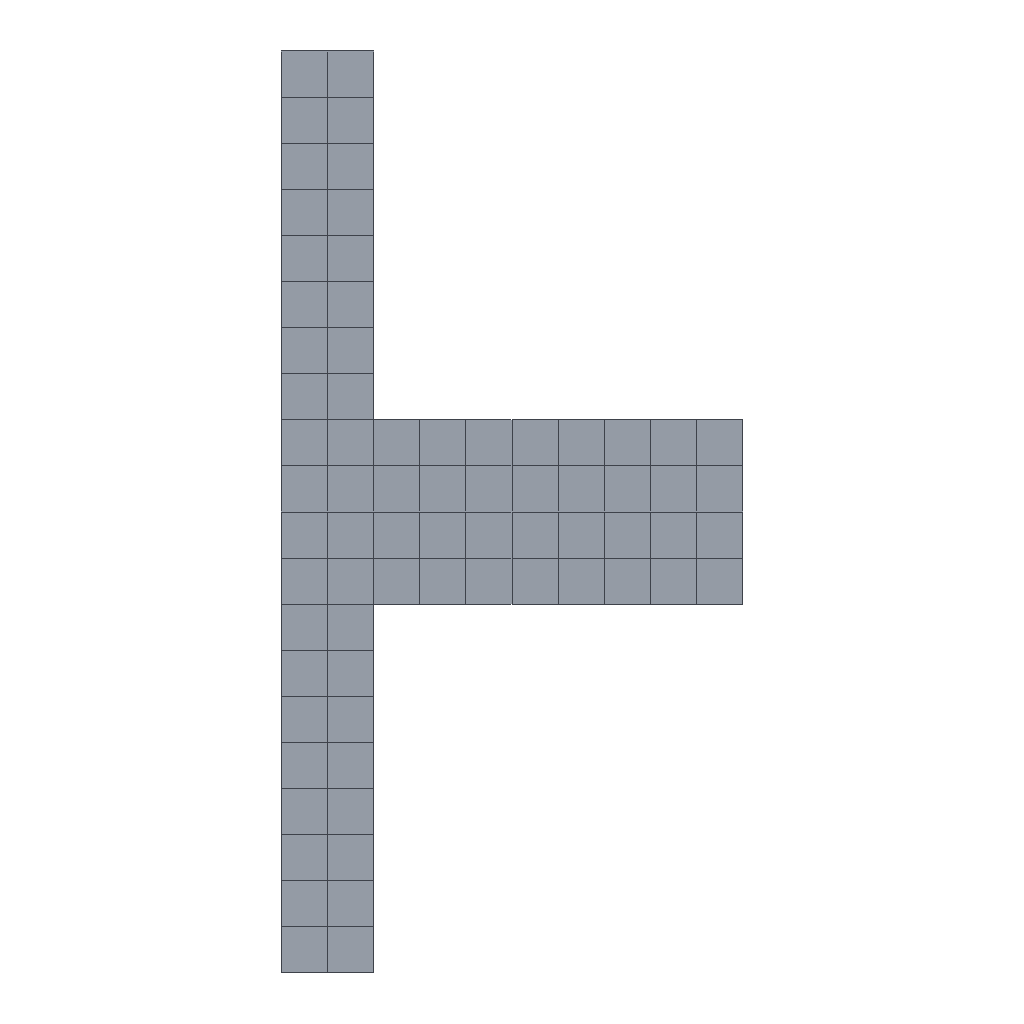Simulation study | abaqus
Set-up summary:
category,name,step,type,value,unit,region
solver,abaqus
solver,version,,,Abaqus/Standard 3DEXPERIENCE R2017x HotFix 2
units,not stated in the deck,,not stated
analysis,deck,,static,static
load_step,deadLoad,deadLoad,static
load_step,heat1,heat1,static
load_step,cool1,cool1,static
load_step,heat2,heat2,static
load_step,cool2,cool2,static
load_step,heat3,heat3,static
load_step,cool3,cool3,static
load_step,heat4,heat4,static
load_step,cool4,cool4,static
load_step,requested,,,9
mesh,nodes,,,114
mesh,elements,,,72
element_type,CAX4I,,axisymmetric,72
load,load commands in deck,,count,10
bc,support commands in deck,,count,2
material,STEEL,,in results
check,setup vs results,,match,"per instance, exact: element labels, types and connectivity; labels of the nodes the elements use; coordinates of those nodes at SINGLE_PRECISION in 2 of 2 instance(s)"
Abaqus input file, long lists of numbers shortened:
*Heading
** Job name: flange_kin Model name: flange_kin
** Generated by: Abaqus/CAE 2017.HF2
*Preprint, echo=NO, model=NO, history=NO, contact=NO
**
** PARTS
**
*Part, name=botFlange
*End Part
**
*Part, name=topFlange
*End Part
**
**
** ASSEMBLY
**
*Assembly, name=Assembly
**
*Instance, name=botFlange-1, part=botFlange
*Node
      1, 0.09, -0.02
      2,  0.13, -0.02
** (55 more lines like these left out)
*Element, type=CAX4I
1,  1, 10, 42,  4
2, 10, 11, 43, 42
** (34 more lines like these left out)
*Nset, nset=_PickedSet2, internal, generate
  1,  57,   1
*Elset, elset=_PickedSet2, internal, generate
  1,  36,   1
** Section: Section-1
*Solid Section, elset=_PickedSet2, material=steel
1.,
*End Instance
**
*Instance, name=topFlange-1, part=topFlange
*Node
      1, 0.09,           0.
      2,  0.13,           0.
** (55 more lines like these left out)
*Element, type=CAX4I
1,  1, 10, 42,  4
2, 10, 11, 43, 42
** (34 more lines like these left out)
*Nset, nset=_PickedSet2, internal, generate
  1,  57,   1
*Elset, elset=_PickedSet2, internal, generate
  1,  36,   1
** Section: Section-1
*Solid Section, elset=_PickedSet2, material=steel
1.,
*End Instance
**
*Nset, nset=all, instance=botFlange-1, generate
  1,  57,   1
*Nset, nset=all, instance=topFlange-1, generate
  1,  57,   1
*Elset, elset=all, instance=botFlange-1, generate
  1,  36,   1
*Elset, elset=all, instance=topFlange-1, generate
  1,  36,   1
*Nset, nset=botBolt, instance=botFlange-1
 4,
*Nset, nset=fix, instance=topFlange-1
 6,
*Nset, nset=topBolt, instance=topFlange-1
 4,
*Nset, nset=tops, instance=botFlange-1
  7,  8, 31
*Nset, nset=tops, instance=topFlange-1
  7,  8, 27
*Elset, elset=tops, instance=botFlange-1
 23, 24
*Elset, elset=tops, instance=topFlange-1
 26, 36
*Elset, elset=_botFlange_S3, internal, instance=botFlange-1
  5,  6,  7,  8, 31, 32, 33, 34, 35, 36
*Surface, type=ELEMENT, name=botFlange
_botFlange_S3, S3
*Elset, elset=_press_S3, internal, instance=botFlange-1
 23, 24
*Elset, elset=_press_S2, internal, instance=topFlange-1
 26, 36
*Surface, type=ELEMENT, name=press
_press_S3, S3
_press_S2, S2
*Elset, elset=_topFlange_S1, internal, instance=topFlange-1, generate
 1,  4,  1
*Elset, elset=_topFlange_S2, internal, instance=topFlange-1, generate
 10,  16,   2
*Elset, elset=_topFlange_S4, internal, instance=topFlange-1
 17, 27
*Surface, type=ELEMENT, name=topFlange
_topFlange_S1, S1
_topFlange_S2, S2
_topFlange_S4, S4
** Constraint: tie bolt 1
*Equation
2
topBolt, 1, 1.
botBolt, 1, -1.
** Constraint: tie bolt 2
*Equation
2
topBolt, 2, 1.
botBolt, 2, -1.
*End Assembly
**
** MATERIALS
**
*Material, name=steel
*Elastic
 2.10439e+11, 0.3
*Expansion
 2e-05,
*Plastic, hardening=KINEMATIC
     2e+08,      0.
 1.237e+09, 0.05411
**
** INTERACTION PROPERTIES
**
*Surface Interaction, name=fric
1.,
*Friction, slip tolerance=0.005
 0.1,
*Surface Behavior, pressure-overclosure=HARD
**
** INTERACTIONS
**
** Interaction: Int-1
*Contact Pair, interaction=fric, small sliding
topFlange, botFlange
** ----------------------------------------------------------------
**
** STEP: deadLoad
**
*Step, name=deadLoad, nlgeom=YES
apply dead load of pipe weight
*Static
0.1, 1., 1e-05, 1.
**
** BOUNDARY CONDITIONS
**
** Name: fixRB Type: Displacement/Rotation
*Boundary
fix, 2, 2
**
** LOADS
**
** Name: Load-1   Type: Pressure
*Dsload
press, P, -4.9735e+07
**
** PREDEFINED FIELDS
**
** Name: Field-1   Type: Temperature
*Temperature
all, 20.
**
** OUTPUT REQUESTS
**
*Restart, write, frequency=0
**
** FIELD OUTPUT: F-Output-1
**
*Output, field, variable=PRESELECT
**
** HISTORY OUTPUT: H-Output-1
**
*Output, history, variable=PRESELECT
*End Step
** ----------------------------------------------------------------
**
** STEP: heat1
**
*Step, name=heat1, nlgeom=YES
1st heat up cycle
*Static
0.05, 1., 1e-05, 1.
**
** BOUNDARY CONDITIONS
**
** Name: fixRB Type: Displacement/Rotation
*Boundary, op=NEW
** Name: fixTops Type: Velocity/Angular velocity
*Boundary, op=NEW, type=VELOCITY
tops, 2, 2
**
** LOADS
**
** Name: Load-1   Type: Pressure
*Dsload, op=NEW
**
** PREDEFINED FIELDS
**
** Name: Field-1   Type: Temperature
*Temperature
all, 350.
**
** OUTPUT REQUESTS
**
*Restart, write, frequency=0
**
** FIELD OUTPUT: F-Output-1
**
*Output, field, variable=PRESELECT
**
** HISTORY OUTPUT: H-Output-1
**
*Output, history, variable=PRESELECT
*End Step
** ----------------------------------------------------------------
**
** STEP: cool1
**
*Step, name=cool1, nlgeom=YES
1st cooling cycle
*Static
0.05, 1., 1e-05, 1.
**
** PREDEFINED FIELDS
**
** Name: Field-1   Type: Temperature
*Temperature
all, 25.
**
** OUTPUT REQUESTS
**
*Restart, write, frequency=0
**
** FIELD OUTPUT: F-Output-1
**
*Output, field, variable=PRESELECT
**
** HISTORY OUTPUT: H-Output-1
**
*Output, history, variable=PRESELECT
*End Step
** ----------------------------------------------------------------
**
** STEP: heat2
**
*Step, name=heat2, nlgeom=YES
2nd heat up cycle
*Static
0.05, 1., 1e-05, 1.
**
** PREDEFINED FIELDS
**
** Name: Field-1   Type: Temperature
*Temperature
all, 350.
**
** OUTPUT REQUESTS
**
*Restart, write, frequency=0
**
** FIELD OUTPUT: F-Output-1
**
*Output, field, variable=PRESELECT
**
** HISTORY OUTPUT: H-Output-1
**
*Output, history, variable=PRESELECT
*End Step
** ----------------------------------------------------------------
**
** STEP: cool2
**
*Step, name=cool2, nlgeom=YES
2nd cooling cycle
*Static
0.05, 1., 1e-05, 1.
**
** PREDEFINED FIELDS
**
** Name: Field-1   Type: Temperature
*Temperature
all, 25.
**
** OUTPUT REQUESTS
**
*Restart, write, frequency=0
**
** FIELD OUTPUT: F-Output-1
**
*Output, field, variable=PRESELECT
**
** HISTORY OUTPUT: H-Output-1
**
*Output, history, variable=PRESELECT
*End Step
** ----------------------------------------------------------------
**
** STEP: heat3
**
*Step, name=heat3, nlgeom=YES
3rd heat up cycle
*Static
0.05, 1., 1e-05, 1.
**
** PREDEFINED FIELDS
**
** Name: Field-1   Type: Temperature
*Temperature
all, 350.
**
** OUTPUT REQUESTS
**
*Restart, write, frequency=0
**
** FIELD OUTPUT: F-Output-1
**
*Output, field, variable=PRESELECT
**
** HISTORY OUTPUT: H-Output-1
**
*Output, history, variable=PRESELECT
*End Step
** ----------------------------------------------------------------
**
** STEP: cool3
**
*Step, name=cool3, nlgeom=YES
3rd cooling cycle
*Static
0.05, 1., 1e-05, 1.
**
** PREDEFINED FIELDS
**
** Name: Field-1   Type: Temperature
*Temperature
all, 25.
**
** OUTPUT REQUESTS
**
*Restart, write, frequency=0
**
** FIELD OUTPUT: F-Output-1
**
*Output, field, variable=PRESELECT
**
** HISTORY OUTPUT: H-Output-1
**
*Output, history, variable=PRESELECT
*End Step
** ----------------------------------------------------------------
**
** STEP: heat4
**
*Step, name=heat4, nlgeom=YES
4th heat up cycle
*Static
0.05, 1., 1e-05, 1.
**
** PREDEFINED FIELDS
**
** Name: Field-1   Type: Temperature
*Temperature
all, 350.
**
** OUTPUT REQUESTS
**
*Restart, write, frequency=0
**
** FIELD OUTPUT: F-Output-1
**
*Output, field, variable=PRESELECT
**
** HISTORY OUTPUT: H-Output-1
**
*Output, history, variable=PRESELECT
*End Step
** ----------------------------------------------------------------
**
** STEP: cool4
**
*Step, name=cool4, nlgeom=YES
4th cooling cycle
*Static
0.05, 1., 1e-05, 1.
**
** PREDEFINED FIELDS
**
** Name: Field-1   Type: Temperature
*Temperature
all, 25.
**
** OUTPUT REQUESTS
**
*Restart, write, frequency=0
**
** FIELD OUTPUT: F-Output-1
**
*Output, field, variable=PRESELECT
**
** HISTORY OUTPUT: H-Output-1
**
*Output, history, variable=PRESELECT
*End Step
Results summary:
result,step,apply dead load of pipe weight,completed,increments=6 time=1.0/1.0
result,step,1st heat up cycle,completed,increments=7 time=1.0/1.0
result,step,1st cooling cycle,completed,increments=7 time=1.0/1.0
result,step,2nd heat up cycle,completed,increments=9 time=1.0/1.0
result,step,2nd cooling cycle,completed,increments=10 time=1.0/1.0
result,step,3rd heat up cycle,completed,increments=9 time=1.0/1.0
result,step,3rd cooling cycle,completed,increments=7 time=1.0/1.0
result,step,4th heat up cycle,completed,increments=9 time=1.0/1.0
result,step,4th cooling cycle,completed,increments=7 time=1.0/1.0
result,analysis,,,static
result,last_loadstep,,,9
result,primary field,,,U
result,reaction total,,FX,0.0,model units
result,reaction total,,FY,0.0,model units
result,reaction total,,FZ,0.0,model units